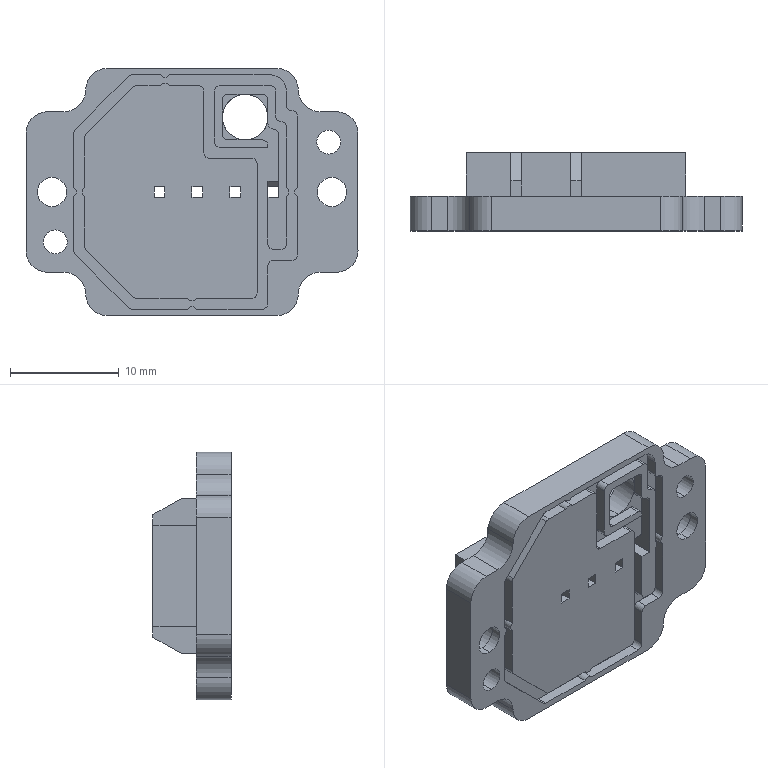Part | STEP file | 30_1_1_1 | 1 solid | 438 faces | box 30.6 x 7.2 x 22.8 mm | volume 1932 mm3 | plane 359 | cylinder 75 | cone 4 | commonest cylinder face diameters 1 x40 4 x12 2.7 x8 3 x5 1.5 x4 2.2 x4